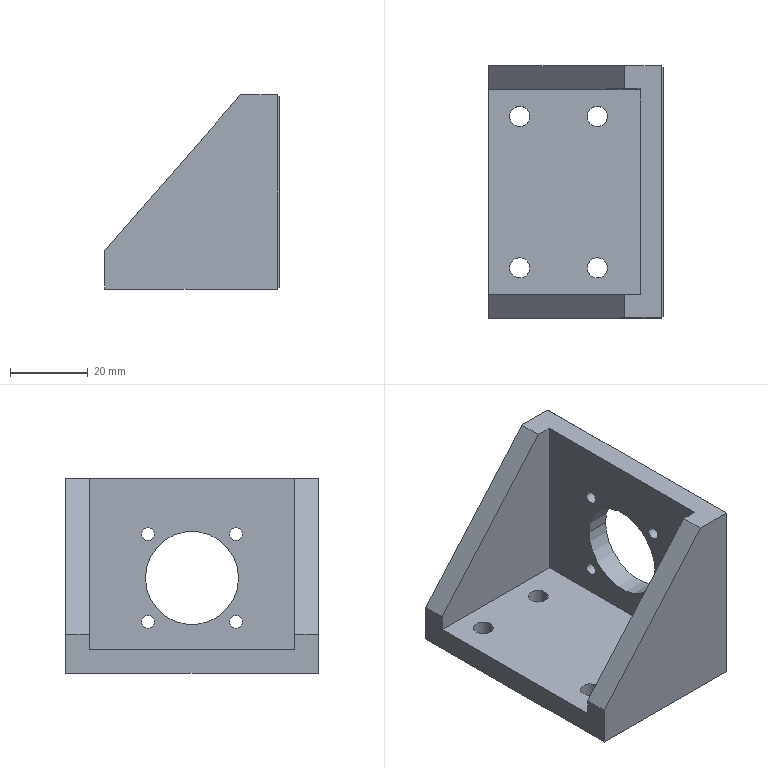Part | Creo | features CURVE 4, CUT 3, DATUM PLANE 3, CHAMFER 1, COORDINATE SYSTEM 1, PROTRUSION 1 | 1 solid | 34 faces | volume 43444 mm3 | cylinder 18 | plane 16 | commonest cylinder face diameters 3.3 x8 5.2 x8 24 x2